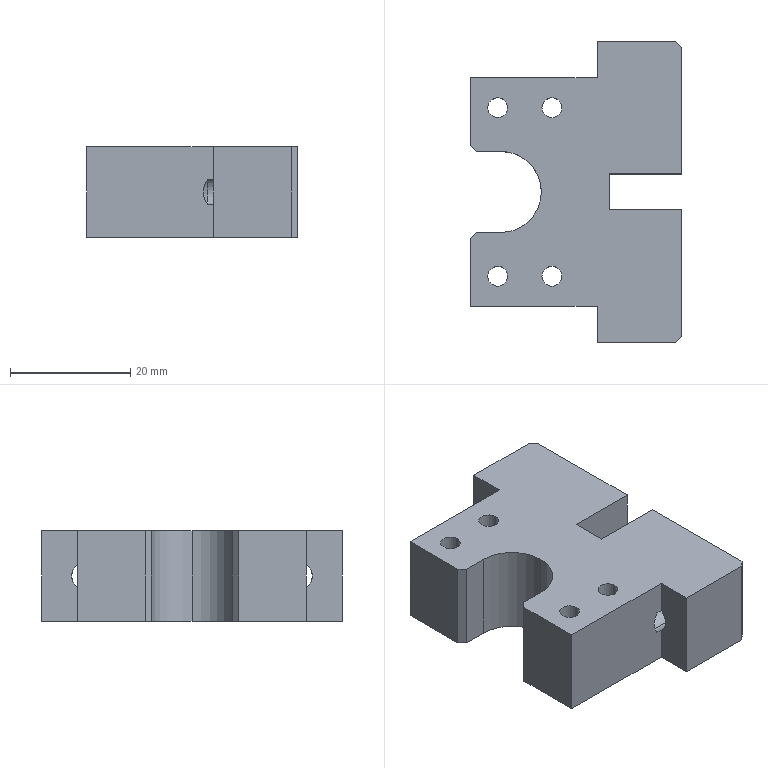Part | SolidWorks | features HoleWzd 3, Chamfer 2, ICE 2, Cut 1, Extrusion 1 | 1 solid | 39 faces | box 35 x 50 x 15 mm | volume 18159 mm3 | plane 21 | cylinder 14 | cone 4 | commonest cylinder face diameters 3.3 x8 5 x4 13.5 x2
STEP:
#1=CARTESIAN_POINT('',(2.5,-17.5,2.5));
#2=VERTEX_POINT('',#1);
#3=CARTESIAN_POINT('',(2.5,-19.,2.));
#4=VERTEX_POINT('',#3);
#5=CARTESIAN_POINT('',(2.5,-17.5,0.));
#6=DIRECTION('',(1.,0.,0.));
#7=DIRECTION('',(0.,0.,-1.));
#8=AXIS2_PLACEMENT_3D('',#5,#6,#7);
#9=CIRCLE('',#8,2.5);
#10=EDGE_CURVE('',#2,#4,#9,.T.);
#11=ORIENTED_EDGE('',*,*,#10,.F.);
#12=CARTESIAN_POINT('',(17.5,-17.5,2.5));
#13=VERTEX_POINT('',#12);
#14=CARTESIAN_POINT('',(17.5,-17.5,2.5));
#15=DIRECTION('',(1.,0.,0.));
#16=VECTOR('',#15,1000.);
#17=LINE('',#14,#16);
#18=EDGE_CURVE('',#2,#13,#17,.T.);
#19=ORIENTED_EDGE('',*,*,#18,.T.);
#20=CARTESIAN_POINT('',(17.5,-17.5,-2.5));
#21=VERTEX_POINT('',#20);
#22=CARTESIAN_POINT('',(17.5,-17.5,0.));
#23=DIRECTION('',(1.,0.,0.));
#24=DIRECTION('',(0.,0.,-1.));
#25=AXIS2_PLACEMENT_3D('',#22,#23,#24);
#26=CIRCLE('',#25,2.5);
#27=EDGE_CURVE('',#13,#21,#26,.T.);
#28=ORIENTED_EDGE('',*,*,#27,.T.);
#29=CARTESIAN_POINT('',(2.5,-17.5,-2.5));
#30=VERTEX_POINT('',#29);
#31=CARTESIAN_POINT('',(17.5,-17.5,-2.5));
#32=DIRECTION('',(1.,0.,0.));
#33=VECTOR('',#32,1000.);
#34=LINE('',#31,#33);
#35=EDGE_CURVE('',#30,#21,#34,.T.);
#36=ORIENTED_EDGE('',*,*,#35,.F.);
#37=CARTESIAN_POINT('',(2.5,-19.,-2.));
#38=VERTEX_POINT('',#37);
#39=CARTESIAN_POINT('',(2.5,-17.5,0.));
#40=DIRECTION('',(1.,0.,0.));
#41=DIRECTION('',(0.,0.,-1.));
#42=AXIS2_PLACEMENT_3D('',#39,#40,#41);
#43=CIRCLE('',#42,2.5);
#44=EDGE_CURVE('',#38,#30,#43,.T.);
#45=ORIENTED_EDGE('',*,*,#44,.F.);
#46=CARTESIAN_POINT('',(3.5,-19.,-2.));
#47=VERTEX_POINT('',#46);
#48=CARTESIAN_POINT('',(17.5,-19.,-2.));
#49=DIRECTION('',(1.,0.,0.));
#50=VECTOR('',#49,1000.);
#51=LINE('',#48,#50);
#52=EDGE_CURVE('',#38,#47,#51,.T.);
#53=ORIENTED_EDGE('',*,*,#52,.T.);
#54=CARTESIAN_POINT('',(3.5,-19.,2.));
#55=VERTEX_POINT('',#54);
#56=CARTESIAN_POINT('',(3.5,-17.5,0.));
#57=DIRECTION('',(-1.,0.,0.));
#58=DIRECTION('',(0.,0.,-1.));
#59=AXIS2_PLACEMENT_3D('',#56,#57,#58);
#60=CIRCLE('',#59,2.5);
#61=EDGE_CURVE('',#47,#55,#60,.T.);
#62=ORIENTED_EDGE('',*,*,#61,.T.);
#63=CARTESIAN_POINT('',(17.5,-19.,2.));
#64=DIRECTION('',(-1.,0.,0.));
#65=VECTOR('',#64,1000.);
#66=LINE('',#63,#65);
#67=EDGE_CURVE('',#55,#4,#66,.T.);
#68=ORIENTED_EDGE('',*,*,#67,.T.);
#69=EDGE_LOOP('',(#11,#19,#28,#36,#45,#53,#62,#68));
#70=FACE_OUTER_BOUND('',#69,.T.);
#71=CARTESIAN_POINT('',(17.5,-17.5,0.));
#72=DIRECTION('',(1.,0.,0.));
#73=DIRECTION('',(0.,0.,-1.));
#74=AXIS2_PLACEMENT_3D('',#71,#72,#73);
#75=CYLINDRICAL_SURFACE('',#74,2.5);
#76=ADVANCED_FACE('',(#70),#75,.F.);
#77=CARTESIAN_POINT('',(0.9978,-17.5,0.));
#78=VERTEX_POINT('',#77);
#79=CARTESIAN_POINT('',(2.5,-17.5,-2.5));
#80=DIRECTION('',(0.515,0.,-0.8572));
#81=VECTOR('',#80,1000.);
#82=LINE('',#79,#81);
#83=EDGE_CURVE('',#78,#30,#82,.T.);
#84=ORIENTED_EDGE('',*,*,#83,.F.);
#85=CARTESIAN_POINT('',(2.5,-17.5,2.5));
#86=DIRECTION('',(0.515,0.,0.8572));
#87=VECTOR('',#86,1000.);
#88=LINE('',#85,#87);
#89=EDGE_CURVE('',#78,#2,#88,.T.);
#90=ORIENTED_EDGE('',*,*,#89,.T.);
#91=ORIENTED_EDGE('',*,*,#10,.T.);
#92=CARTESIAN_POINT('',(2.5,-19.,2.));
#93=CARTESIAN_POINT('',(2.348,-19.,1.683));
#94=CARTESIAN_POINT('',(2.204,-19.,1.361));
#95=CARTESIAN_POINT('',(1.978,-19.,0.6968));
#96=CARTESIAN_POINT('',(1.899,-19.,0.3477));
#97=CARTESIAN_POINT('',(1.899,-19.,-0.1759));
#98=CARTESIAN_POINT('',(1.919,-19.,-0.3531));
#99=CARTESIAN_POINT('',(1.987,-19.,-0.698));
#100=CARTESIAN_POINT('',(2.035,-19.,-0.866));
#101=CARTESIAN_POINT('',(2.204,-19.,-1.362));
#102=CARTESIAN_POINT('',(2.348,-19.,-1.684));
#103=CARTESIAN_POINT('',(2.5,-19.,-2.));
#104=B_SPLINE_CURVE_WITH_KNOTS('',3,(#92,#93,#94,#95,#96,#97,#98,#99,#100,#101,#102,#103),.UNSPECIFIED.,.F.,.F.,(4,2,2,2,2,4),(0.006568,0.007624,0.008679,0.009206,0.009734,0.01079),.UNSPECIFIED.);
#105=EDGE_CURVE('',#4,#38,#104,.T.);
#106=ORIENTED_EDGE('',*,*,#105,.T.);
#107=ORIENTED_EDGE('',*,*,#44,.T.);
#108=EDGE_LOOP('',(#84,#90,#91,#106,#107));
#109=FACE_OUTER_BOUND('',#108,.T.);
#110=CARTESIAN_POINT('',(2.5,-17.5,0.));
#111=DIRECTION('',(1.,0.,0.));
#112=DIRECTION('',(0.,0.,-1.));
#113=AXIS2_PLACEMENT_3D('',#110,#111,#112);
#114=CONICAL_SURFACE('',#113,2.5,1.03);
#115=ADVANCED_FACE('',(#109),#114,.F.);
#116=CARTESIAN_POINT('',(2.5,17.5,2.5));
#117=VERTEX_POINT('',#116);
#118=CARTESIAN_POINT('',(2.5,17.5,-2.5));
#119=VERTEX_POINT('',#118);
#120=CARTESIAN_POINT('',(2.5,17.5,0.));
#121=DIRECTION('',(1.,0.,0.));
#122=DIRECTION('',(0.,0.,-1.));
#123=AXIS2_PLACEMENT_3D('',#120,#121,#122);
#124=CIRCLE('',#123,2.5);
#125=EDGE_CURVE('',#117,#119,#124,.T.);
#126=ORIENTED_EDGE('',*,*,#125,.F.);
#127=CARTESIAN_POINT('',(17.5,17.5,2.5));
#128=VERTEX_POINT('',#127);
#129=CARTESIAN_POINT('',(17.5,17.5,2.5));
#130=DIRECTION('',(1.,0.,0.));
#131=VECTOR('',#130,1000.);
#132=LINE('',#129,#131);
#133=EDGE_CURVE('',#117,#128,#132,.T.);
#134=ORIENTED_EDGE('',*,*,#133,.T.);
#135=CARTESIAN_POINT('',(17.5,17.5,-2.5));
#136=VERTEX_POINT('',#135);
#137=CARTESIAN_POINT('',(17.5,17.5,0.));
#138=DIRECTION('',(1.,0.,0.));
#139=DIRECTION('',(0.,0.,-1.));
#140=AXIS2_PLACEMENT_3D('',#137,#138,#139);
#141=CIRCLE('',#140,2.5);
#142=EDGE_CURVE('',#128,#136,#141,.T.);
#143=ORIENTED_EDGE('',*,*,#142,.T.);
#144=CARTESIAN_POINT('',(17.5,17.5,-2.5));
#145=DIRECTION('',(1.,0.,0.));
#146=VECTOR('',#145,1000.);
#147=LINE('',#144,#146);
#148=EDGE_CURVE('',#119,#136,#147,.T.);
#149=ORIENTED_EDGE('',*,*,#148,.F.);
#150=EDGE_LOOP('',(#126,#134,#143,#149));
#151=FACE_OUTER_BOUND('',#150,.T.);
#152=CARTESIAN_POINT('',(17.5,17.5,0.));
#153=DIRECTION('',(1.,0.,0.));
#154=DIRECTION('',(0.,0.,-1.));
#155=AXIS2_PLACEMENT_3D('',#152,#153,#154);
#156=CYLINDRICAL_SURFACE('',#155,2.5);
#157=ADVANCED_FACE('',(#151),#156,.F.);
#158=CARTESIAN_POINT('',(0.9978,17.5,0.));
#159=VERTEX_POINT('',#158);
#160=CARTESIAN_POINT('',(2.5,17.5,-2.5));
#161=DIRECTION('',(0.515,0.,-0.8572));
#162=VECTOR('',#161,1000.);
#163=LINE('',#160,#162);
#164=EDGE_CURVE('',#159,#119,#163,.T.);
#165=ORIENTED_EDGE('',*,*,#164,.F.);
#166=CARTESIAN_POINT('',(2.5,17.5,2.5));
#167=DIRECTION('',(0.515,0.,0.8572));
#168=VECTOR('',#167,1000.);
#169=LINE('',#166,#168);
#170=EDGE_CURVE('',#159,#117,#169,.T.);
#171=ORIENTED_EDGE('',*,*,#170,.T.);
#172=ORIENTED_EDGE('',*,*,#125,.T.);
#173=EDGE_LOOP('',(#165,#171,#172));
#174=FACE_OUTER_BOUND('',#173,.T.);
#175=CARTESIAN_POINT('',(2.5,17.5,0.));
#176=DIRECTION('',(1.,0.,0.));
#177=DIRECTION('',(0.,0.,-1.));
#178=AXIS2_PLACEMENT_3D('',#175,#176,#177);
#179=CONICAL_SURFACE('',#178,2.5,1.03);
#180=ADVANCED_FACE('',(#174),#179,.F.);
#181=CARTESIAN_POINT('',(-2.35,-14.,7.5));
#182=VERTEX_POINT('',#181);
#183=CARTESIAN_POINT('',(-5.65,-14.,7.5));
#184=VERTEX_POINT('',#183);
#185=CARTESIAN_POINT('',(-4.,-14.,7.5));
#186=DIRECTION('',(0.,0.,-1.));
#187=DIRECTION('',(-1.,0.,0.));
#188=AXIS2_PLACEMENT_3D('',#185,#186,#187);
#189=CIRCLE('',#188,1.65);
#190=EDGE_CURVE('',#182,#184,#189,.T.);
#191=ORIENTED_EDGE('',*,*,#190,.F.);
#192=CARTESIAN_POINT('',(-2.35,-14.,-7.5));
#193=VERTEX_POINT('',#192);
#194=CARTESIAN_POINT('',(-2.35,-14.,-7.5));
#195=DIRECTION('',(0.,0.,-1.));
#196=VECTOR('',#195,1000.);
#197=LINE('',#194,#196);
#198=EDGE_CURVE('',#182,#193,#197,.T.);
#199=ORIENTED_EDGE('',*,*,#198,.T.);
#200=CARTESIAN_POINT('',(-5.65,-14.,-7.5));
#201=VERTEX_POINT('',#200);
#202=CARTESIAN_POINT('',(-4.,-14.,-7.5));
#203=DIRECTION('',(0.,0.,-1.));
#204=DIRECTION('',(-1.,0.,0.));
#205=AXIS2_PLACEMENT_3D('',#202,#203,#204);
#206=CIRCLE('',#205,1.65);
#207=EDGE_CURVE('',#193,#201,#206,.T.);
#208=ORIENTED_EDGE('',*,*,#207,.T.);
#209=CARTESIAN_POINT('',(-5.65,-14.,-7.5));
#210=DIRECTION('',(0.,0.,-1.));
#211=VECTOR('',#210,1000.);
#212=LINE('',#209,#211);
#213=EDGE_CURVE('',#184,#201,#212,.T.);
#214=ORIENTED_EDGE('',*,*,#213,.F.);
#215=EDGE_LOOP('',(#191,#199,#208,#214));
#216=FACE_OUTER_BOUND('',#215,.T.);
#217=CARTESIAN_POINT('',(-4.,-14.,-7.5));
#218=DIRECTION('',(0.,0.,-1.));
#219=DIRECTION('',(-1.,0.,0.));
#220=AXIS2_PLACEMENT_3D('',#217,#218,#219);
#221=CYLINDRICAL_SURFACE('',#220,1.65);
#222=ADVANCED_FACE('',(#216),#221,.F.);
#223=CARTESIAN_POINT('',(-11.35,-14.,7.5));
#224=VERTEX_POINT('',#223);
#225=CARTESIAN_POINT('',(-14.65,-14.,7.5));
#226=VERTEX_POINT('',#225);
#227=CARTESIAN_POINT('',(-13.,-14.,7.5));
#228=DIRECTION('',(0.,0.,-1.));
#229=DIRECTION('',(-1.,0.,0.));
#230=AXIS2_PLACEMENT_3D('',#227,#228,#229);
#231=CIRCLE('',#230,1.65);
#232=EDGE_CURVE('',#224,#226,#231,.T.);
#233=ORIENTED_EDGE('',*,*,#232,.F.);
#234=CARTESIAN_POINT('',(-11.35,-14.,-7.5));
#235=VERTEX_POINT('',#234);
#236=CARTESIAN_POINT('',(-11.35,-14.,-7.5));
#237=DIRECTION('',(0.,0.,-1.));
#238=VECTOR('',#237,1000.);
#239=LINE('',#236,#238);
#240=EDGE_CURVE('',#224,#235,#239,.T.);
#241=ORIENTED_EDGE('',*,*,#240,.T.);
#242=CARTESIAN_POINT('',(-14.65,-14.,-7.5));
#243=VERTEX_POINT('',#242);
#244=CARTESIAN_POINT('',(-13.,-14.,-7.5));
#245=DIRECTION('',(0.,0.,-1.));
#246=DIRECTION('',(-1.,0.,0.));
#247=AXIS2_PLACEMENT_3D('',#244,#245,#246);
#248=CIRCLE('',#247,1.65);
#249=EDGE_CURVE('',#235,#243,#248,.T.);
#250=ORIENTED_EDGE('',*,*,#249,.T.);
#251=CARTESIAN_POINT('',(-14.65,-14.,-7.5));
#252=DIRECTION('',(0.,0.,-1.));
#253=VECTOR('',#252,1000.);
#254=LINE('',#251,#253);
#255=EDGE_CURVE('',#226,#243,#254,.T.);
#256=ORIENTED_EDGE('',*,*,#255,.F.);
#257=EDGE_LOOP('',(#233,#241,#250,#256));
#258=FACE_OUTER_BOUND('',#257,.T.);
#259=CARTESIAN_POINT('',(-13.,-14.,-7.5));
#260=DIRECTION('',(0.,0.,-1.));
#261=DIRECTION('',(-1.,0.,0.));
#262=AXIS2_PLACEMENT_3D('',#259,#260,#261);
#263=CYLINDRICAL_SURFACE('',#262,1.65);
#264=ADVANCED_FACE('',(#258),#263,.F.);
#265=CARTESIAN_POINT('',(-2.35,14.,7.5));
#266=VERTEX_POINT('',#265);
#267=CARTESIAN_POINT('',(-5.65,14.,7.5));
#268=VERTEX_POINT('',#267);
#269=CARTESIAN_POINT('',(-4.,14.,7.5));
#270=DIRECTION('',(0.,0.,-1.));
#271=DIRECTION('',(-1.,0.,0.));
#272=AXIS2_PLACEMENT_3D('',#269,#270,#271);
#273=CIRCLE('',#272,1.65);
#274=EDGE_CURVE('',#266,#268,#273,.T.);
#275=ORIENTED_EDGE('',*,*,#274,.F.);
#276=CARTESIAN_POINT('',(-2.35,14.,-7.5));
#277=VERTEX_POINT('',#276);
#278=CARTESIAN_POINT('',(-2.35,14.,-7.5));
#279=DIRECTION('',(0.,0.,-1.));
#280=VECTOR('',#279,1000.);
#281=LINE('',#278,#280);
#282=EDGE_CURVE('',#266,#277,#281,.T.);
#283=ORIENTED_EDGE('',*,*,#282,.T.);
#284=CARTESIAN_POINT('',(-5.65,14.,-7.5));
#285=VERTEX_POINT('',#284);
#286=CARTESIAN_POINT('',(-4.,14.,-7.5));
#287=DIRECTION('',(0.,0.,-1.));
#288=DIRECTION('',(-1.,0.,0.));
#289=AXIS2_PLACEMENT_3D('',#286,#287,#288);
#290=CIRCLE('',#289,1.65);
#291=EDGE_CURVE('',#277,#285,#290,.T.);
#292=ORIENTED_EDGE('',*,*,#291,.T.);
#293=CARTESIAN_POINT('',(-5.65,14.,-7.5));
#294=DIRECTION('',(0.,0.,-1.));
#295=VECTOR('',#294,1000.);
#296=LINE('',#293,#295);
#297=EDGE_CURVE('',#268,#285,#296,.T.);
#298=ORIENTED_EDGE('',*,*,#297,.F.);
#299=EDGE_LOOP('',(#275,#283,#292,#298));
#300=FACE_OUTER_BOUND('',#299,.T.);
#301=CARTESIAN_POINT('',(-4.,14.,-7.5));
#302=DIRECTION('',(0.,0.,-1.));
#303=DIRECTION('',(-1.,0.,0.));
#304=AXIS2_PLACEMENT_3D('',#301,#302,#303);
#305=CYLINDRICAL_SURFACE('',#304,1.65);
#306=ADVANCED_FACE('',(#300),#305,.F.);
#307=CARTESIAN_POINT('',(-11.35,14.,7.5));
#308=VERTEX_POINT('',#307);
#309=CARTESIAN_POINT('',(-14.65,14.,7.5));
#310=VERTEX_POINT('',#309);
#311=CARTESIAN_POINT('',(-13.,14.,7.5));
#312=DIRECTION('',(0.,0.,-1.));
#313=DIRECTION('',(-1.,0.,0.));
#314=AXIS2_PLACEMENT_3D('',#311,#312,#313);
#315=CIRCLE('',#314,1.65);
#316=EDGE_CURVE('',#308,#310,#315,.T.);
#317=ORIENTED_EDGE('',*,*,#316,.F.);
#318=CARTESIAN_POINT('',(-11.35,14.,-7.5));
#319=VERTEX_POINT('',#318);
#320=CARTESIAN_POINT('',(-11.35,14.,-7.5));
#321=DIRECTION('',(0.,0.,-1.));
#322=VECTOR('',#321,1000.);
#323=LINE('',#320,#322);
#324=EDGE_CURVE('',#308,#319,#323,.T.);
#325=ORIENTED_EDGE('',*,*,#324,.T.);
#326=CARTESIAN_POINT('',(-14.65,14.,-7.5));
#327=VERTEX_POINT('',#326);
#328=CARTESIAN_POINT('',(-13.,14.,-7.5));
#329=DIRECTION('',(0.,0.,-1.));
#330=DIRECTION('',(-1.,0.,0.));
#331=AXIS2_PLACEMENT_3D('',#328,#329,#330);
#332=CIRCLE('',#331,1.65);
#333=EDGE_CURVE('',#319,#327,#332,.T.);
#334=ORIENTED_EDGE('',*,*,#333,.T.);
#335=CARTESIAN_POINT('',(-14.65,14.,-7.5));
#336=DIRECTION('',(0.,0.,-1.));
#337=VECTOR('',#336,1000.);
#338=LINE('',#335,#337);
#339=EDGE_CURVE('',#310,#327,#338,.T.);
#340=ORIENTED_EDGE('',*,*,#339,.F.);
#341=EDGE_LOOP('',(#317,#325,#334,#340));
#342=FACE_OUTER_BOUND('',#341,.T.);
#343=CARTESIAN_POINT('',(-13.,14.,-7.5));
#344=DIRECTION('',(0.,0.,-1.));
#345=DIRECTION('',(-1.,0.,0.));
#346=AXIS2_PLACEMENT_3D('',#343,#344,#345);
#347=CYLINDRICAL_SURFACE('',#346,1.65);
#348=ADVANCED_FACE('',(#342),#347,.F.);
#349=CARTESIAN_POINT('',(-5.75,0.,-7.5));
#350=VERTEX_POINT('',#349);
#351=CARTESIAN_POINT('',(-12.5,6.75,-7.5));
#352=VERTEX_POINT('',#351);
#353=CARTESIAN_POINT('',(-12.5,0.,-7.5));
#354=DIRECTION('',(0.,0.,1.));
#355=DIRECTION('',(1.,0.,0.));
#356=AXIS2_PLACEMENT_3D('',#353,#354,#355);
#357=CIRCLE('',#356,6.75);
#358=EDGE_CURVE('',#350,#352,#357,.T.);
#359=ORIENTED_EDGE('',*,*,#358,.F.);
#360=CARTESIAN_POINT('',(-5.75,0.,7.5));
#361=VERTEX_POINT('',#360);
#362=CARTESIAN_POINT('',(-5.75,0.,-7.5));
#363=DIRECTION('',(0.,0.,1.));
#364=VECTOR('',#363,1000.);
#365=LINE('',#362,#364);
#366=EDGE_CURVE('',#350,#361,#365,.T.);
#367=ORIENTED_EDGE('',*,*,#366,.T.);
#368=CARTESIAN_POINT('',(-12.5,6.75,7.5));
#369=VERTEX_POINT('',#368);
#370=CARTESIAN_POINT('',(-12.5,0.,7.5));
#371=DIRECTION('',(0.,0.,1.));
#372=DIRECTION('',(1.,0.,0.));
#373=AXIS2_PLACEMENT_3D('',#370,#371,#372);
#374=CIRCLE('',#373,6.75);
#375=EDGE_CURVE('',#361,#369,#374,.T.);
#376=ORIENTED_EDGE('',*,*,#375,.T.);
#377=CARTESIAN_POINT('',(-12.5,6.75,-7.5));
#378=DIRECTION('',(0.,0.,1.));
#379=VECTOR('',#378,1000.);
#380=LINE('',#377,#379);
#381=EDGE_CURVE('',#352,#369,#380,.T.);
#382=ORIENTED_EDGE('',*,*,#381,.F.);
#383=EDGE_LOOP('',(#359,#367,#376,#382));
#384=FACE_OUTER_BOUND('',#383,.T.);
#385=CARTESIAN_POINT('',(-12.5,0.,-7.5));
#386=DIRECTION('',(0.,0.,1.));
#387=DIRECTION('',(1.,0.,0.));
#388=AXIS2_PLACEMENT_3D('',#385,#386,#387);
#389=CYLINDRICAL_SURFACE('',#388,6.75);
#390=ADVANCED_FACE('',(#384),#389,.F.);
#391=CARTESIAN_POINT('',(17.5,-17.5,0.));
#392=DIRECTION('',(1.,0.,0.));
#393=DIRECTION('',(0.,0.,-1.));
#394=AXIS2_PLACEMENT_3D('',#391,#392,#393);
#395=CIRCLE('',#394,2.5);
#396=EDGE_CURVE('',#21,#13,#395,.T.);
#397=ORIENTED_EDGE('',*,*,#396,.F.);
#398=ORIENTED_EDGE('',*,*,#27,.F.);
#399=EDGE_LOOP('',(#397,#398));
#400=FACE_BOUND('',#399,.T.);
#401=CARTESIAN_POINT('',(17.5,-24.,-7.5));
#402=VERTEX_POINT('',#401);
#403=CARTESIAN_POINT('',(17.5,-3.,-7.5));
#404=VERTEX_POINT('',#403);
#405=CARTESIAN_POINT('',(17.5,-25.,-7.5));
#406=DIRECTION('',(0.,1.,0.));
#407=VECTOR('',#406,1000.);
#408=LINE('',#405,#407);
#409=EDGE_CURVE('',#402,#404,#408,.T.);
#410=ORIENTED_EDGE('',*,*,#409,.T.);
#411=CARTESIAN_POINT('',(17.5,-3.,7.5));
#412=VERTEX_POINT('',#411);
#413=CARTESIAN_POINT('',(17.5,-3.,-7.5));
#414=DIRECTION('',(0.,0.,1.));
#415=VECTOR('',#414,1000.);
#416=LINE('',#413,#415);
#417=EDGE_CURVE('',#404,#412,#416,.T.);
#418=ORIENTED_EDGE('',*,*,#417,.T.);
#419=CARTESIAN_POINT('',(17.5,-24.,7.5));
#420=VERTEX_POINT('',#419);
#421=CARTESIAN_POINT('',(17.5,-25.,7.5));
#422=DIRECTION('',(0.,1.,0.));
#423=VECTOR('',#422,1000.);
#424=LINE('',#421,#423);
#425=EDGE_CURVE('',#420,#412,#424,.T.);
#426=ORIENTED_EDGE('',*,*,#425,.F.);
#427=CARTESIAN_POINT('',(17.5,-24.,7.5));
#428=DIRECTION('',(0.,0.,-1.));
#429=VECTOR('',#428,1000.);
#430=LINE('',#427,#429);
#431=EDGE_CURVE('',#420,#402,#430,.T.);
#432=ORIENTED_EDGE('',*,*,#431,.T.);
#433=EDGE_LOOP('',(#410,#418,#426,#432));
#434=FACE_OUTER_BOUND('',#433,.T.);
#435=CARTESIAN_POINT('',(17.5,-25.,7.5));
#436=DIRECTION('',(-1.,0.,0.));
#437=DIRECTION('',(0.,0.,1.));
#438=AXIS2_PLACEMENT_3D('',#435,#436,#437);
#439=PLANE('',#438);
#440=ADVANCED_FACE('',(#400,#434),#439,.F.);
#441=CARTESIAN_POINT('',(-17.5,19.,7.5));
#442=VERTEX_POINT('',#441);
#443=CARTESIAN_POINT('',(-17.5,7.75,7.5));
#444=VERTEX_POINT('',#443);
#445=CARTESIAN_POINT('',(-17.5,-25.,7.5));
#446=DIRECTION('',(0.,-1.,0.));
#447=VECTOR('',#446,1000.);
#448=LINE('',#445,#447);
#449=EDGE_CURVE('',#442,#444,#448,.T.);
#450=ORIENTED_EDGE('',*,*,#449,.F.);
#451=CARTESIAN_POINT('',(-17.5,19.,-7.5));
#452=VERTEX_POINT('',#451);
#453=CARTESIAN_POINT('',(-17.5,19.,-7.5));
#454=DIRECTION('',(0.,0.,1.));
#455=VECTOR('',#454,1000.);
#456=LINE('',#453,#455);
#457=EDGE_CURVE('',#452,#442,#456,.T.);
#458=ORIENTED_EDGE('',*,*,#457,.F.);
#459=CARTESIAN_POINT('',(-17.5,7.75,-7.5));
#460=VERTEX_POINT('',#459);
#461=CARTESIAN_POINT('',(-17.5,-25.,-7.5));
#462=DIRECTION('',(0.,-1.,0.));
#463=VECTOR('',#462,1000.);
#464=LINE('',#461,#463);
#465=EDGE_CURVE('',#452,#460,#464,.T.);
#466=ORIENTED_EDGE('',*,*,#465,.T.);
#467=CARTESIAN_POINT('',(-17.5,7.75,7.5));
#468=DIRECTION('',(0.,0.,1.));
#469=VECTOR('',#468,1000.);
#470=LINE('',#467,#469);
#471=EDGE_CURVE('',#460,#444,#470,.T.);
#472=ORIENTED_EDGE('',*,*,#471,.T.);
#473=EDGE_LOOP('',(#450,#458,#466,#472));
#474=FACE_OUTER_BOUND('',#473,.T.);
#475=CARTESIAN_POINT('',(-17.5,-25.,7.5));
#476=DIRECTION('',(1.,0.,0.));
#477=DIRECTION('',(0.,0.,-1.));
#478=AXIS2_PLACEMENT_3D('',#475,#476,#477);
#479=PLANE('',#478);
#480=ADVANCED_FACE('',(#474),#479,.F.);
#481=CARTESIAN_POINT('',(17.5,17.5,0.));
#482=DIRECTION('',(1.,0.,0.));
#483=DIRECTION('',(0.,0.,-1.));
#484=AXIS2_PLACEMENT_3D('',#481,#482,#483);
#485=CIRCLE('',#484,2.5);
#486=EDGE_CURVE('',#136,#128,#485,.T.);
#487=ORIENTED_EDGE('',*,*,#486,.F.);
#488=ORIENTED_EDGE('',*,*,#142,.F.);
#489=EDGE_LOOP('',(#487,#488));
#490=FACE_BOUND('',#489,.T.);
#491=CARTESIAN_POINT('',(17.5,3.,7.5));
#492=VERTEX_POINT('',#491);
#493=CARTESIAN_POINT('',(17.5,24.,7.5));
#494=VERTEX_POINT('',#493);
#495=CARTESIAN_POINT('',(17.5,-25.,7.5));
#496=DIRECTION('',(0.,1.,0.));
#497=VECTOR('',#496,1000.);
#498=LINE('',#495,#497);
#499=EDGE_CURVE('',#492,#494,#498,.T.);
#500=ORIENTED_EDGE('',*,*,#499,.F.);
#501=CARTESIAN_POINT('',(17.5,3.,-7.5));
#502=VERTEX_POINT('',#501);
#503=CARTESIAN_POINT('',(17.5,3.,-7.5));
#504=DIRECTION('',(0.,0.,1.));
#505=VECTOR('',#504,1000.);
#506=LINE('',#503,#505);
#507=EDGE_CURVE('',#502,#492,#506,.T.);
#508=ORIENTED_EDGE('',*,*,#507,.F.);
#509=CARTESIAN_POINT('',(17.5,24.,-7.5));
#510=VERTEX_POINT('',#509);
#511=CARTESIAN_POINT('',(17.5,-25.,-7.5));
#512=DIRECTION('',(0.,1.,0.));
#513=VECTOR('',#512,1000.);
#514=LINE('',#511,#513);
#515=EDGE_CURVE('',#502,#510,#514,.T.);
#516=ORIENTED_EDGE('',*,*,#515,.T.);
#517=CARTESIAN_POINT('',(17.5,24.,7.5));
#518=DIRECTION('',(0.,0.,1.));
#519=VECTOR('',#518,1000.);
#520=LINE('',#517,#519);
#521=EDGE_CURVE('',#510,#494,#520,.T.);
#522=ORIENTED_EDGE('',*,*,#521,.T.);
#523=EDGE_LOOP('',(#500,#508,#516,#522));
#524=FACE_OUTER_BOUND('',#523,.T.);
#525=CARTESIAN_POINT('',(17.5,-25.,7.5));
#526=DIRECTION('',(-1.,0.,0.));
#527=DIRECTION('',(0.,0.,1.));
#528=AXIS2_PLACEMENT_3D('',#525,#526,#527);
#529=PLANE('',#528);
#530=ADVANCED_FACE('',(#490,#524),#529,.F.);
#531=CARTESIAN_POINT('',(16.5,25.,-7.5));
#532=VERTEX_POINT('',#531);
#533=CARTESIAN_POINT('',(3.5,25.,-7.5));
#534=VERTEX_POINT('',#533);
#535=CARTESIAN_POINT('',(-17.5,25.,-7.5));
#536=DIRECTION('',(-1.,0.,0.));
#537=VECTOR('',#536,1000.);
#538=LINE('',#535,#537);
#539=EDGE_CURVE('',#532,#534,#538,.T.);
#540=ORIENTED_EDGE('',*,*,#539,.T.);
#541=CARTESIAN_POINT('',(3.5,25.,7.5));
#542=VERTEX_POINT('',#541);
#543=CARTESIAN_POINT('',(3.5,25.,-7.5));
#544=DIRECTION('',(0.,0.,1.));
#545=VECTOR('',#544,1000.);
#546=LINE('',#543,#545);
#547=EDGE_CURVE('',#534,#542,#546,.T.);
#548=ORIENTED_EDGE('',*,*,#547,.T.);
#549=CARTESIAN_POINT('',(16.5,25.,7.5));
#550=VERTEX_POINT('',#549);
#551=CARTESIAN_POINT('',(-17.5,25.,7.5));
#552=DIRECTION('',(-1.,0.,0.));
#553=VECTOR('',#552,1000.);
#554=LINE('',#551,#553);
#555=EDGE_CURVE('',#550,#542,#554,.T.);
#556=ORIENTED_EDGE('',*,*,#555,.F.);
#557=CARTESIAN_POINT('',(16.5,25.,7.5));
#558=DIRECTION('',(0.,0.,-1.));
#559=VECTOR('',#558,1000.);
#560=LINE('',#557,#559);
#561=EDGE_CURVE('',#550,#532,#560,.T.);
#562=ORIENTED_EDGE('',*,*,#561,.T.);
#563=EDGE_LOOP('',(#540,#548,#556,#562));
#564=FACE_OUTER_BOUND('',#563,.T.);
#565=CARTESIAN_POINT('',(-17.5,25.,7.5));
#566=DIRECTION('',(0.,-1.,0.));
#567=DIRECTION('',(0.,0.,-1.));
#568=AXIS2_PLACEMENT_3D('',#565,#566,#567);
#569=PLANE('',#568);
#570=ADVANCED_FACE('',(#564),#569,.F.);
#571=CARTESIAN_POINT('',(-17.5,-7.75,-7.5));
#572=VERTEX_POINT('',#571);
#573=CARTESIAN_POINT('',(-17.5,-19.,-7.5));
#574=VERTEX_POINT('',#573);
#575=CARTESIAN_POINT('',(-17.5,-25.,-7.5));
#576=DIRECTION('',(0.,-1.,0.));
#577=VECTOR('',#576,1000.);
#578=LINE('',#575,#577);
#579=EDGE_CURVE('',#572,#574,#578,.T.);
#580=ORIENTED_EDGE('',*,*,#579,.T.);
#581=CARTESIAN_POINT('',(-17.5,-19.,7.5));
#582=VERTEX_POINT('',#581);
#583=CARTESIAN_POINT('',(-17.5,-19.,-7.5));
#584=DIRECTION('',(0.,0.,1.));
#585=VECTOR('',#584,1000.);
#586=LINE('',#583,#585);
#587=EDGE_CURVE('',#574,#582,#586,.T.);
#588=ORIENTED_EDGE('',*,*,#587,.T.);
#589=CARTESIAN_POINT('',(-17.5,-7.75,7.5));
#590=VERTEX_POINT('',#589);
#591=CARTESIAN_POINT('',(-17.5,-25.,7.5));
#592=DIRECTION('',(0.,-1.,0.));
#593=VECTOR('',#592,1000.);
#594=LINE('',#591,#593);
#595=EDGE_CURVE('',#590,#582,#594,.T.);
#596=ORIENTED_EDGE('',*,*,#595,.F.);
#597=CARTESIAN_POINT('',(-17.5,-7.75,7.5));
#598=DIRECTION('',(0.,0.,-1.));
#599=VECTOR('',#598,1000.);
#600=LINE('',#597,#599);
#601=EDGE_CURVE('',#590,#572,#600,.T.);
#602=ORIENTED_EDGE('',*,*,#601,.T.);
#603=EDGE_LOOP('',(#580,#588,#596,#602));
#604=FACE_OUTER_BOUND('',#603,.T.);
#605=CARTESIAN_POINT('',(-17.5,-25.,7.5));
#606=DIRECTION('',(1.,0.,0.));
#607=DIRECTION('',(0.,0.,-1.));
#608=AXIS2_PLACEMENT_3D('',#605,#606,#607);
#609=PLANE('',#608);
#610=ADVANCED_FACE('',(#604),#609,.F.);
#611=CARTESIAN_POINT('',(3.5,-25.,7.5));
#612=VERTEX_POINT('',#611);
#613=CARTESIAN_POINT('',(16.5,-25.,7.5));
#614=VERTEX_POINT('',#613);
#615=CARTESIAN_POINT('',(-17.5,-25.,7.5));
#616=DIRECTION('',(1.,0.,0.));
#617=VECTOR('',#616,1000.);
#618=LINE('',#615,#617);
#619=EDGE_CURVE('',#612,#614,#618,.T.);
#620=ORIENTED_EDGE('',*,*,#619,.F.);
#621=CARTESIAN_POINT('',(3.5,-25.,-7.5));
#622=VERTEX_POINT('',#621);
#623=CARTESIAN_POINT('',(3.5,-25.,-7.5));
#624=DIRECTION('',(0.,0.,1.));
#625=VECTOR('',#624,1000.);
#626=LINE('',#623,#625);
#627=EDGE_CURVE('',#622,#612,#626,.T.);
#628=ORIENTED_EDGE('',*,*,#627,.F.);
#629=CARTESIAN_POINT('',(16.5,-25.,-7.5));
#630=VERTEX_POINT('',#629);
#631=CARTESIAN_POINT('',(-17.5,-25.,-7.5));
#632=DIRECTION('',(1.,0.,0.));
#633=VECTOR('',#632,1000.);
#634=LINE('',#631,#633);
#635=EDGE_CURVE('',#622,#630,#634,.T.);
#636=ORIENTED_EDGE('',*,*,#635,.T.);
#637=CARTESIAN_POINT('',(16.5,-25.,7.5));
#638=DIRECTION('',(0.,0.,1.));
#639=VECTOR('',#638,1000.);
#640=LINE('',#637,#639);
#641=EDGE_CURVE('',#630,#614,#640,.T.);
#642=ORIENTED_EDGE('',*,*,#641,.T.);
#643=EDGE_LOOP('',(#620,#628,#636,#642));
#644=FACE_OUTER_BOUND('',#643,.T.);
#645=CARTESIAN_POINT('',(-17.5,-25.,7.5));
#646=DIRECTION('',(0.,1.,0.));
#647=DIRECTION('',(0.,0.,1.));
#648=AXIS2_PLACEMENT_3D('',#645,#646,#647);
#649=PLANE('',#648);
#650=ADVANCED_FACE('',(#644),#649,.F.);
#651=CARTESIAN_POINT('',(-4.,-14.,7.5));
#652=DIRECTION('',(0.,0.,-1.));
#653=DIRECTION('',(-1.,0.,0.));
#654=AXIS2_PLACEMENT_3D('',#651,#652,#653);
#655=CIRCLE('',#654,1.65);
#656=EDGE_CURVE('',#184,#182,#655,.T.);
#657=ORIENTED_EDGE('',*,*,#656,.T.);
#658=ORIENTED_EDGE('',*,*,#190,.T.);
#659=EDGE_LOOP('',(#657,#658));
#660=FACE_BOUND('',#659,.T.);
#661=CARTESIAN_POINT('',(-13.,-14.,7.5));
#662=DIRECTION('',(0.,0.,-1.));
#663=DIRECTION('',(-1.,0.,0.));
#664=AXIS2_PLACEMENT_3D('',#661,#662,#663);
#665=CIRCLE('',#664,1.65);
#666=EDGE_CURVE('',#226,#224,#665,.T.);
#667=ORIENTED_EDGE('',*,*,#666,.T.);
#668=ORIENTED_EDGE('',*,*,#232,.T.);
#669=EDGE_LOOP('',(#667,#668));
#670=FACE_BOUND('',#669,.T.);
#671=CARTESIAN_POINT('',(-4.,14.,7.5));
#672=DIRECTION('',(0.,0.,-1.));
#673=DIRECTION('',(-1.,0.,0.));
#674=AXIS2_PLACEMENT_3D('',#671,#672,#673);
#675=CIRCLE('',#674,1.65);
#676=EDGE_CURVE('',#268,#266,#675,.T.);
#677=ORIENTED_EDGE('',*,*,#676,.T.);
#678=ORIENTED_EDGE('',*,*,#274,.T.);
#679=EDGE_LOOP('',(#677,#678));
#680=FACE_BOUND('',#679,.T.);
#681=CARTESIAN_POINT('',(-13.,14.,7.5));
#682=DIRECTION('',(0.,0.,-1.));
#683=DIRECTION('',(-1.,0.,0.));
#684=AXIS2_PLACEMENT_3D('',#681,#682,#683);
#685=CIRCLE('',#684,1.65);
#686=EDGE_CURVE('',#310,#308,#685,.T.);
#687=ORIENTED_EDGE('',*,*,#686,.T.);
#688=ORIENTED_EDGE('',*,*,#316,.T.);
#689=EDGE_LOOP('',(#687,#688));
#690=FACE_BOUND('',#689,.T.);
#691=ORIENTED_EDGE('',*,*,#595,.T.);
#692=CARTESIAN_POINT('',(3.5,-19.,7.5));
#693=VERTEX_POINT('',#692);
#694=CARTESIAN_POINT('',(-17.5,-19.,7.5));
#695=DIRECTION('',(-1.,0.,0.));
#696=VECTOR('',#695,1000.);
#697=LINE('',#694,#696);
#698=EDGE_CURVE('',#693,#582,#697,.T.);
#699=ORIENTED_EDGE('',*,*,#698,.F.);
#700=CARTESIAN_POINT('',(3.5,-25.,7.5));
#701=DIRECTION('',(0.,1.,0.));
#702=VECTOR('',#701,1000.);
#703=LINE('',#700,#702);
#704=EDGE_CURVE('',#612,#693,#703,.T.);
#705=ORIENTED_EDGE('',*,*,#704,.F.);
#706=ORIENTED_EDGE('',*,*,#619,.T.);
#707=CARTESIAN_POINT('',(17.5,-24.,7.5));
#708=DIRECTION('',(0.7071,0.7071,0.));
#709=VECTOR('',#708,1000.);
#710=LINE('',#707,#709);
#711=EDGE_CURVE('',#614,#420,#710,.T.);
#712=ORIENTED_EDGE('',*,*,#711,.T.);
#713=ORIENTED_EDGE('',*,*,#425,.T.);
#714=CARTESIAN_POINT('',(5.5,-3.,7.5));
#715=VERTEX_POINT('',#714);
#716=CARTESIAN_POINT('',(5.5,-3.,7.5));
#717=DIRECTION('',(1.,0.,0.));
#718=VECTOR('',#717,1000.);
#719=LINE('',#716,#718);
#720=EDGE_CURVE('',#715,#412,#719,.T.);
#721=ORIENTED_EDGE('',*,*,#720,.F.);
#722=CARTESIAN_POINT('',(5.5,3.,7.5));
#723=VERTEX_POINT('',#722);
#724=CARTESIAN_POINT('',(5.5,3.,7.5));
#725=DIRECTION('',(0.,-1.,0.));
#726=VECTOR('',#725,1000.);
#727=LINE('',#724,#726);
#728=EDGE_CURVE('',#723,#715,#727,.T.);
#729=ORIENTED_EDGE('',*,*,#728,.F.);
#730=CARTESIAN_POINT('',(5.5,3.,7.5));
#731=DIRECTION('',(-1.,0.,0.));
#732=VECTOR('',#731,1000.);
#733=LINE('',#730,#732);
#734=EDGE_CURVE('',#492,#723,#733,.T.);
#735=ORIENTED_EDGE('',*,*,#734,.F.);
#736=ORIENTED_EDGE('',*,*,#499,.T.);
#737=CARTESIAN_POINT('',(16.5,25.,7.5));
#738=DIRECTION('',(-0.7071,0.7071,0.));
#739=VECTOR('',#738,1000.);
#740=LINE('',#737,#739);
#741=EDGE_CURVE('',#494,#550,#740,.T.);
#742=ORIENTED_EDGE('',*,*,#741,.T.);
#743=ORIENTED_EDGE('',*,*,#555,.T.);
#744=CARTESIAN_POINT('',(3.5,19.,7.5));
#745=VERTEX_POINT('',#744);
#746=CARTESIAN_POINT('',(3.5,19.,7.5));
#747=DIRECTION('',(0.,1.,0.));
#748=VECTOR('',#747,1000.);
#749=LINE('',#746,#748);
#750=EDGE_CURVE('',#745,#542,#749,.T.);
#751=ORIENTED_EDGE('',*,*,#750,.F.);
#752=CARTESIAN_POINT('',(-17.5,19.,7.5));
#753=DIRECTION('',(1.,0.,0.));
#754=VECTOR('',#753,1000.);
#755=LINE('',#752,#754);
#756=EDGE_CURVE('',#442,#745,#755,.T.);
#757=ORIENTED_EDGE('',*,*,#756,.F.);
#758=ORIENTED_EDGE('',*,*,#449,.T.);
#759=CARTESIAN_POINT('',(-16.5,6.75,7.5));
#760=VERTEX_POINT('',#759);
#761=CARTESIAN_POINT('',(-17.5,7.75,7.5));
#762=DIRECTION('',(0.7071,-0.7071,0.));
#763=VECTOR('',#762,1000.);
#764=LINE('',#761,#763);
#765=EDGE_CURVE('',#444,#760,#764,.T.);
#766=ORIENTED_EDGE('',*,*,#765,.T.);
#767=CARTESIAN_POINT('',(-17.5,6.75,7.5));
#768=DIRECTION('',(-1.,0.,0.));
#769=VECTOR('',#768,1000.);
#770=LINE('',#767,#769);
#771=EDGE_CURVE('',#369,#760,#770,.T.);
#772=ORIENTED_EDGE('',*,*,#771,.F.);
#773=ORIENTED_EDGE('',*,*,#375,.F.);
#774=CARTESIAN_POINT('',(-12.5,-6.75,7.5));
#775=VERTEX_POINT('',#774);
#776=CARTESIAN_POINT('',(-12.5,0.,7.5));
#777=DIRECTION('',(0.,0.,1.));
#778=DIRECTION('',(1.,0.,0.));
#779=AXIS2_PLACEMENT_3D('',#776,#777,#778);
#780=CIRCLE('',#779,6.75);
#781=EDGE_CURVE('',#775,#361,#780,.T.);
#782=ORIENTED_EDGE('',*,*,#781,.F.);
#783=CARTESIAN_POINT('',(-16.5,-6.75,7.5));
#784=VERTEX_POINT('',#783);
#785=CARTESIAN_POINT('',(-17.5,-6.75,7.5));
#786=DIRECTION('',(1.,0.,0.));
#787=VECTOR('',#786,1000.);
#788=LINE('',#785,#787);
#789=EDGE_CURVE('',#784,#775,#788,.T.);
#790=ORIENTED_EDGE('',*,*,#789,.F.);
#791=CARTESIAN_POINT('',(-16.5,-6.75,7.5));
#792=DIRECTION('',(-0.7071,-0.7071,0.));
#793=VECTOR('',#792,1000.);
#794=LINE('',#791,#793);
#795=EDGE_CURVE('',#784,#590,#794,.T.);
#796=ORIENTED_EDGE('',*,*,#795,.T.);
#797=EDGE_LOOP('',(#691,#699,#705,#706,#712,#713,#721,#729,#735,#736,#742,#743,#751,#757,#758,#766,#772,#773,#782,#790,#796));
#798=FACE_OUTER_BOUND('',#797,.T.);
#799=CARTESIAN_POINT('',(0.,0.,7.5));
#800=DIRECTION('',(0.,0.,-1.));
#801=DIRECTION('',(-1.,0.,0.));
#802=AXIS2_PLACEMENT_3D('',#799,#800,#801);
#803=PLANE('',#802);
#804=ADVANCED_FACE('',(#660,#670,#680,#690,#798),#803,.F.);
#805=CARTESIAN_POINT('',(3.5,-19.,-7.5));
#806=VERTEX_POINT('',#805);
#807=CARTESIAN_POINT('',(-17.5,-19.,-7.5));
#808=DIRECTION('',(-1.,0.,0.));
#809=VECTOR('',#808,1000.);
#810=LINE('',#807,#809);
#811=EDGE_CURVE('',#806,#574,#810,.T.);
#812=ORIENTED_EDGE('',*,*,#811,.T.);
#813=ORIENTED_EDGE('',*,*,#579,.F.);
#814=CARTESIAN_POINT('',(-16.5,-6.75,-7.5));
#815=VERTEX_POINT('',#814);
#816=CARTESIAN_POINT('',(-4.875,4.875,-7.5));
#817=DIRECTION('',(0.7071,0.7071,0.));
#818=VECTOR('',#817,1000.);
#819=LINE('',#816,#818);
#820=EDGE_CURVE('',#572,#815,#819,.T.);
#821=ORIENTED_EDGE('',*,*,#820,.T.);
#822=CARTESIAN_POINT('',(-12.5,-6.75,-7.5));
#823=VERTEX_POINT('',#822);
#824=CARTESIAN_POINT('',(-17.5,-6.75,-7.5));
#825=DIRECTION('',(1.,0.,0.));
#826=VECTOR('',#825,1000.);
#827=LINE('',#824,#826);
#828=EDGE_CURVE('',#815,#823,#827,.T.);
#829=ORIENTED_EDGE('',*,*,#828,.T.);
#830=CARTESIAN_POINT('',(-12.5,0.,-7.5));
#831=DIRECTION('',(0.,0.,1.));
#832=DIRECTION('',(1.,0.,0.));
#833=AXIS2_PLACEMENT_3D('',#830,#831,#832);
#834=CIRCLE('',#833,6.75);
#835=EDGE_CURVE('',#823,#350,#834,.T.);
#836=ORIENTED_EDGE('',*,*,#835,.T.);
#837=ORIENTED_EDGE('',*,*,#358,.T.);
#838=CARTESIAN_POINT('',(-16.5,6.75,-7.5));
#839=VERTEX_POINT('',#838);
#840=CARTESIAN_POINT('',(-17.5,6.75,-7.5));
#841=DIRECTION('',(-1.,0.,0.));
#842=VECTOR('',#841,1000.);
#843=LINE('',#840,#842);
#844=EDGE_CURVE('',#352,#839,#843,.T.);
#845=ORIENTED_EDGE('',*,*,#844,.T.);
#846=CARTESIAN_POINT('',(-4.875,-4.875,-7.5));
#847=DIRECTION('',(-0.7071,0.7071,0.));
#848=VECTOR('',#847,1000.);
#849=LINE('',#846,#848);
#850=EDGE_CURVE('',#839,#460,#849,.T.);
#851=ORIENTED_EDGE('',*,*,#850,.T.);
#852=ORIENTED_EDGE('',*,*,#465,.F.);
#853=CARTESIAN_POINT('',(3.5,19.,-7.5));
#854=VERTEX_POINT('',#853);
#855=CARTESIAN_POINT('',(-17.5,19.,-7.5));
#856=DIRECTION('',(1.,0.,0.));
#857=VECTOR('',#856,1000.);
#858=LINE('',#855,#857);
#859=EDGE_CURVE('',#452,#854,#858,.T.);
#860=ORIENTED_EDGE('',*,*,#859,.T.);
#861=CARTESIAN_POINT('',(3.5,19.,-7.5));
#862=DIRECTION('',(0.,1.,0.));
#863=VECTOR('',#862,1000.);
#864=LINE('',#861,#863);
#865=EDGE_CURVE('',#854,#534,#864,.T.);
#866=ORIENTED_EDGE('',*,*,#865,.T.);
#867=ORIENTED_EDGE('',*,*,#539,.F.);
#868=CARTESIAN_POINT('',(20.75,20.75,-7.5));
#869=DIRECTION('',(0.7071,-0.7071,0.));
#870=VECTOR('',#869,1000.);
#871=LINE('',#868,#870);
#872=EDGE_CURVE('',#532,#510,#871,.T.);
#873=ORIENTED_EDGE('',*,*,#872,.T.);
#874=ORIENTED_EDGE('',*,*,#515,.F.);
#875=CARTESIAN_POINT('',(5.5,3.,-7.5));
#876=VERTEX_POINT('',#875);
#877=CARTESIAN_POINT('',(5.5,3.,-7.5));
#878=DIRECTION('',(-1.,0.,0.));
#879=VECTOR('',#878,1000.);
#880=LINE('',#877,#879);
#881=EDGE_CURVE('',#502,#876,#880,.T.);
#882=ORIENTED_EDGE('',*,*,#881,.T.);
#883=CARTESIAN_POINT('',(5.5,-3.,-7.5));
#884=VERTEX_POINT('',#883);
#885=CARTESIAN_POINT('',(5.5,3.,-7.5));
#886=DIRECTION('',(0.,-1.,0.));
#887=VECTOR('',#886,1000.);
#888=LINE('',#885,#887);
#889=EDGE_CURVE('',#876,#884,#888,.T.);
#890=ORIENTED_EDGE('',*,*,#889,.T.);
#891=CARTESIAN_POINT('',(5.5,-3.,-7.5));
#892=DIRECTION('',(1.,0.,0.));
#893=VECTOR('',#892,1000.);
#894=LINE('',#891,#893);
#895=EDGE_CURVE('',#884,#404,#894,.T.);
#896=ORIENTED_EDGE('',*,*,#895,.T.);
#897=ORIENTED_EDGE('',*,*,#409,.F.);
#898=CARTESIAN_POINT('',(20.75,-20.75,-7.5));
#899=DIRECTION('',(-0.7071,-0.7071,0.));
#900=VECTOR('',#899,1000.);
#901=LINE('',#898,#900);
#902=EDGE_CURVE('',#402,#630,#901,.T.);
#903=ORIENTED_EDGE('',*,*,#902,.T.);
#904=ORIENTED_EDGE('',*,*,#635,.F.);
#905=CARTESIAN_POINT('',(3.5,-25.,-7.5));
#906=DIRECTION('',(0.,1.,0.));
#907=VECTOR('',#906,1000.);
#908=LINE('',#905,#907);
#909=EDGE_CURVE('',#622,#806,#908,.T.);
#910=ORIENTED_EDGE('',*,*,#909,.T.);
#911=EDGE_LOOP('',(#812,#813,#821,#829,#836,#837,#845,#851,#852,#860,#866,#867,#873,#874,#882,#890,#896,#897,#903,#904,#910));
#912=FACE_OUTER_BOUND('',#911,.T.);
#913=CARTESIAN_POINT('',(-4.,-14.,-7.5));
#914=DIRECTION('',(0.,0.,-1.));
#915=DIRECTION('',(-1.,0.,0.));
#916=AXIS2_PLACEMENT_3D('',#913,#914,#915);
#917=CIRCLE('',#916,1.65);
#918=EDGE_CURVE('',#201,#193,#917,.T.);
#919=ORIENTED_EDGE('',*,*,#918,.F.);
#920=ORIENTED_EDGE('',*,*,#207,.F.);
#921=EDGE_LOOP('',(#919,#920));
#922=FACE_BOUND('',#921,.T.);
#923=CARTESIAN_POINT('',(-13.,-14.,-7.5));
#924=DIRECTION('',(0.,0.,-1.));
#925=DIRECTION('',(-1.,0.,0.));
#926=AXIS2_PLACEMENT_3D('',#923,#924,#925);
#927=CIRCLE('',#926,1.65);
#928=EDGE_CURVE('',#243,#235,#927,.T.);
#929=ORIENTED_EDGE('',*,*,#928,.F.);
#930=ORIENTED_EDGE('',*,*,#249,.F.);
#931=EDGE_LOOP('',(#929,#930));
#932=FACE_BOUND('',#931,.T.);
#933=CARTESIAN_POINT('',(-4.,14.,-7.5));
#934=DIRECTION('',(0.,0.,-1.));
#935=DIRECTION('',(-1.,0.,0.));
#936=AXIS2_PLACEMENT_3D('',#933,#934,#935);
#937=CIRCLE('',#936,1.65);
#938=EDGE_CURVE('',#285,#277,#937,.T.);
#939=ORIENTED_EDGE('',*,*,#938,.F.);
#940=ORIENTED_EDGE('',*,*,#291,.F.);
#941=EDGE_LOOP('',(#939,#940));
#942=FACE_BOUND('',#941,.T.);
#943=CARTESIAN_POINT('',(-13.,14.,-7.5));
#944=DIRECTION('',(0.,0.,-1.));
#945=DIRECTION('',(-1.,0.,0.));
#946=AXIS2_PLACEMENT_3D('',#943,#944,#945);
#947=CIRCLE('',#946,1.65);
#948=EDGE_CURVE('',#327,#319,#947,.T.);
#949=ORIENTED_EDGE('',*,*,#948,.F.);
#950=ORIENTED_EDGE('',*,*,#333,.F.);
#951=EDGE_LOOP('',(#949,#950));
#952=FACE_BOUND('',#951,.T.);
#953=CARTESIAN_POINT('',(0.,0.,-7.5));
#954=DIRECTION('',(0.,0.,-1.));
#955=DIRECTION('',(-1.,0.,0.));
#956=AXIS2_PLACEMENT_3D('',#953,#954,#955);
#957=PLANE('',#956);
#958=ADVANCED_FACE('',(#912,#922,#932,#942,#952),#957,.T.);
#959=ORIENTED_EDGE('',*,*,#771,.T.);
#960=CARTESIAN_POINT('',(-16.5,6.75,-7.5));
#961=DIRECTION('',(0.,0.,-1.));
#962=VECTOR('',#961,1000.);
#963=LINE('',#960,#962);
#964=EDGE_CURVE('',#760,#839,#963,.T.);
#965=ORIENTED_EDGE('',*,*,#964,.T.);
#966=ORIENTED_EDGE('',*,*,#844,.F.);
#967=ORIENTED_EDGE('',*,*,#381,.T.);
#968=EDGE_LOOP('',(#959,#965,#966,#967));
#969=FACE_OUTER_BOUND('',#968,.T.);
#970=CARTESIAN_POINT('',(-17.5,6.75,-7.5));
#971=DIRECTION('',(0.,1.,0.));
#972=DIRECTION('',(0.,0.,1.));
#973=AXIS2_PLACEMENT_3D('',#970,#971,#972);
#974=PLANE('',#973);
#975=ADVANCED_FACE('',(#969),#974,.F.);
#976=ORIENTED_EDGE('',*,*,#366,.F.);
#977=ORIENTED_EDGE('',*,*,#835,.F.);
#978=CARTESIAN_POINT('',(-12.5,-6.75,-7.5));
#979=DIRECTION('',(0.,0.,1.));
#980=VECTOR('',#979,1000.);
#981=LINE('',#978,#980);
#982=EDGE_CURVE('',#823,#775,#981,.T.);
#983=ORIENTED_EDGE('',*,*,#982,.T.);
#984=ORIENTED_EDGE('',*,*,#781,.T.);
#985=EDGE_LOOP('',(#976,#977,#983,#984));
#986=FACE_OUTER_BOUND('',#985,.T.);
#987=CARTESIAN_POINT('',(-12.5,0.,-7.5));
#988=DIRECTION('',(0.,0.,1.));
#989=DIRECTION('',(1.,0.,0.));
#990=AXIS2_PLACEMENT_3D('',#987,#988,#989);
#991=CYLINDRICAL_SURFACE('',#990,6.75);
#992=ADVANCED_FACE('',(#986),#991,.F.);
#993=ORIENTED_EDGE('',*,*,#828,.F.);
#994=CARTESIAN_POINT('',(-16.5,-6.75,-7.5));
#995=DIRECTION('',(0.,0.,1.));
#996=VECTOR('',#995,1000.);
#997=LINE('',#994,#996);
#998=EDGE_CURVE('',#815,#784,#997,.T.);
#999=ORIENTED_EDGE('',*,*,#998,.T.);
#1000=ORIENTED_EDGE('',*,*,#789,.T.);
#1001=ORIENTED_EDGE('',*,*,#982,.F.);
#1002=EDGE_LOOP('',(#993,#999,#1000,#1001));
#1003=FACE_OUTER_BOUND('',#1002,.T.);
#1004=CARTESIAN_POINT('',(-17.5,-6.75,-7.5));
#1005=DIRECTION('',(0.,-1.,0.));
#1006=DIRECTION('',(0.,0.,-1.));
#1007=AXIS2_PLACEMENT_3D('',#1004,#1005,#1006);
#1008=PLANE('',#1007);
#1009=ADVANCED_FACE('',(#1003),#1008,.F.);
#1010=ORIENTED_EDGE('',*,*,#324,.F.);
#1011=ORIENTED_EDGE('',*,*,#686,.F.);
#1012=ORIENTED_EDGE('',*,*,#339,.T.);
#1013=ORIENTED_EDGE('',*,*,#948,.T.);
#1014=EDGE_LOOP('',(#1010,#1011,#1012,#1013));
#1015=FACE_OUTER_BOUND('',#1014,.T.);
#1016=CARTESIAN_POINT('',(-13.,14.,-7.5));
#1017=DIRECTION('',(0.,0.,-1.));
#1018=DIRECTION('',(-1.,0.,0.));
#1019=AXIS2_PLACEMENT_3D('',#1016,#1017,#1018);
#1020=CYLINDRICAL_SURFACE('',#1019,1.65);
#1021=ADVANCED_FACE('',(#1015),#1020,.F.);
#1022=ORIENTED_EDGE('',*,*,#282,.F.);
#1023=ORIENTED_EDGE('',*,*,#676,.F.);
#1024=ORIENTED_EDGE('',*,*,#297,.T.);
#1025=ORIENTED_EDGE('',*,*,#938,.T.);
#1026=EDGE_LOOP('',(#1022,#1023,#1024,#1025));
#1027=FACE_OUTER_BOUND('',#1026,.T.);
#1028=CARTESIAN_POINT('',(-4.,14.,-7.5));
#1029=DIRECTION('',(0.,0.,-1.));
#1030=DIRECTION('',(-1.,0.,0.));
#1031=AXIS2_PLACEMENT_3D('',#1028,#1029,#1030);
#1032=CYLINDRICAL_SURFACE('',#1031,1.65);
#1033=ADVANCED_FACE('',(#1027),#1032,.F.);
#1034=ORIENTED_EDGE('',*,*,#240,.F.);
#1035=ORIENTED_EDGE('',*,*,#666,.F.);
#1036=ORIENTED_EDGE('',*,*,#255,.T.);
#1037=ORIENTED_EDGE('',*,*,#928,.T.);
#1038=EDGE_LOOP('',(#1034,#1035,#1036,#1037));
#1039=FACE_OUTER_BOUND('',#1038,.T.);
#1040=CARTESIAN_POINT('',(-13.,-14.,-7.5));
#1041=DIRECTION('',(0.,0.,-1.));
#1042=DIRECTION('',(-1.,0.,0.));
#1043=AXIS2_PLACEMENT_3D('',#1040,#1041,#1042);
#1044=CYLINDRICAL_SURFACE('',#1043,1.65);
#1045=ADVANCED_FACE('',(#1039),#1044,.F.);
#1046=ORIENTED_EDGE('',*,*,#198,.F.);
#1047=ORIENTED_EDGE('',*,*,#656,.F.);
#1048=ORIENTED_EDGE('',*,*,#213,.T.);
#1049=ORIENTED_EDGE('',*,*,#918,.T.);
#1050=EDGE_LOOP('',(#1046,#1047,#1048,#1049));
#1051=FACE_OUTER_BOUND('',#1050,.T.);
#1052=CARTESIAN_POINT('',(-4.,-14.,-7.5));
#1053=DIRECTION('',(0.,0.,-1.));
#1054=DIRECTION('',(-1.,0.,0.));
#1055=AXIS2_PLACEMENT_3D('',#1052,#1053,#1054);
#1056=CYLINDRICAL_SURFACE('',#1055,1.65);
#1057=ADVANCED_FACE('',(#1051),#1056,.F.);
#1058=ORIENTED_EDGE('',*,*,#741,.F.);
#1059=ORIENTED_EDGE('',*,*,#521,.F.);
#1060=ORIENTED_EDGE('',*,*,#872,.F.);
#1061=ORIENTED_EDGE('',*,*,#561,.F.);
#1062=EDGE_LOOP('',(#1058,#1059,#1060,#1061));
#1063=FACE_OUTER_BOUND('',#1062,.T.);
#1064=CARTESIAN_POINT('',(16.5,25.,7.5));
#1065=DIRECTION('',(-0.7071,-0.7071,0.));
#1066=DIRECTION('',(0.,0.,-1.));
#1067=AXIS2_PLACEMENT_3D('',#1064,#1065,#1066);
#1068=PLANE('',#1067);
#1069=ADVANCED_FACE('',(#1063),#1068,.F.);
#1070=ORIENTED_EDGE('',*,*,#711,.F.);
#1071=ORIENTED_EDGE('',*,*,#641,.F.);
#1072=ORIENTED_EDGE('',*,*,#902,.F.);
#1073=ORIENTED_EDGE('',*,*,#431,.F.);
#1074=EDGE_LOOP('',(#1070,#1071,#1072,#1073));
#1075=FACE_OUTER_BOUND('',#1074,.T.);
#1076=CARTESIAN_POINT('',(17.5,-24.,7.5));
#1077=DIRECTION('',(-0.7071,0.7071,0.));
#1078=DIRECTION('',(0.,0.,-1.));
#1079=AXIS2_PLACEMENT_3D('',#1076,#1077,#1078);
#1080=PLANE('',#1079);
#1081=ADVANCED_FACE('',(#1075),#1080,.F.);
#1082=ORIENTED_EDGE('',*,*,#820,.F.);
#1083=ORIENTED_EDGE('',*,*,#601,.F.);
#1084=ORIENTED_EDGE('',*,*,#795,.F.);
#1085=ORIENTED_EDGE('',*,*,#998,.F.);
#1086=EDGE_LOOP('',(#1082,#1083,#1084,#1085));
#1087=FACE_OUTER_BOUND('',#1086,.T.);
#1088=CARTESIAN_POINT('',(-16.5,-6.75,-7.5));
#1089=DIRECTION('',(0.7071,-0.7071,0.));
#1090=DIRECTION('',(0.,0.,1.));
#1091=AXIS2_PLACEMENT_3D('',#1088,#1089,#1090);
#1092=PLANE('',#1091);
#1093=ADVANCED_FACE('',(#1087),#1092,.F.);
#1094=ORIENTED_EDGE('',*,*,#850,.F.);
#1095=ORIENTED_EDGE('',*,*,#964,.F.);
#1096=ORIENTED_EDGE('',*,*,#765,.F.);
#1097=ORIENTED_EDGE('',*,*,#471,.F.);
#1098=EDGE_LOOP('',(#1094,#1095,#1096,#1097));
#1099=FACE_OUTER_BOUND('',#1098,.T.);
#1100=CARTESIAN_POINT('',(-17.5,7.75,7.5));
#1101=DIRECTION('',(0.7071,0.7071,0.));
#1102=DIRECTION('',(0.,0.,1.));
#1103=AXIS2_PLACEMENT_3D('',#1100,#1101,#1102);
#1104=PLANE('',#1103);
#1105=ADVANCED_FACE('',(#1099),#1104,.F.);
#1106=ORIENTED_EDGE('',*,*,#170,.F.);
#1107=ORIENTED_EDGE('',*,*,#164,.T.);
#1108=CARTESIAN_POINT('',(2.5,19.,-2.));
#1109=VERTEX_POINT('',#1108);
#1110=CARTESIAN_POINT('',(2.5,17.5,0.));
#1111=DIRECTION('',(1.,0.,0.));
#1112=DIRECTION('',(0.,0.,-1.));
#1113=AXIS2_PLACEMENT_3D('',#1110,#1111,#1112);
#1114=CIRCLE('',#1113,2.5);
#1115=EDGE_CURVE('',#119,#1109,#1114,.T.);
#1116=ORIENTED_EDGE('',*,*,#1115,.T.);
#1117=CARTESIAN_POINT('',(2.5,19.,2.));
#1118=VERTEX_POINT('',#1117);
#1119=CARTESIAN_POINT('',(2.5,19.,-2.));
#1120=CARTESIAN_POINT('',(2.348,19.,-1.683));
#1121=CARTESIAN_POINT('',(2.204,19.,-1.361));
#1122=CARTESIAN_POINT('',(1.978,19.,-0.6968));
#1123=CARTESIAN_POINT('',(1.899,19.,-0.3477));
#1124=CARTESIAN_POINT('',(1.899,19.,0.1759));
#1125=CARTESIAN_POINT('',(1.919,19.,0.3531));
#1126=CARTESIAN_POINT('',(1.987,19.,0.698));
#1127=CARTESIAN_POINT('',(2.035,19.,0.866));
#1128=CARTESIAN_POINT('',(2.204,19.,1.362));
#1129=CARTESIAN_POINT('',(2.348,19.,1.684));
#1130=CARTESIAN_POINT('',(2.5,19.,2.));
#1131=B_SPLINE_CURVE_WITH_KNOTS('',3,(#1119,#1120,#1121,#1122,#1123,#1124,#1125,#1126,#1127,#1128,#1129,#1130),.UNSPECIFIED.,.F.,.F.,(4,2,2,2,2,4),(0.006568,0.007624,0.008679,0.009206,0.009734,0.01079),.UNSPECIFIED.);
#1132=EDGE_CURVE('',#1109,#1118,#1131,.T.);
#1133=ORIENTED_EDGE('',*,*,#1132,.T.);
#1134=CARTESIAN_POINT('',(2.5,17.5,0.));
#1135=DIRECTION('',(1.,0.,0.));
#1136=DIRECTION('',(0.,0.,-1.));
#1137=AXIS2_PLACEMENT_3D('',#1134,#1135,#1136);
#1138=CIRCLE('',#1137,2.5);
#1139=EDGE_CURVE('',#1118,#117,#1138,.T.);
#1140=ORIENTED_EDGE('',*,*,#1139,.T.);
#1141=EDGE_LOOP('',(#1106,#1107,#1116,#1133,#1140));
#1142=FACE_OUTER_BOUND('',#1141,.T.);
#1143=CARTESIAN_POINT('',(2.5,17.5,0.));
#1144=DIRECTION('',(1.,0.,0.));
#1145=DIRECTION('',(0.,0.,-1.));
#1146=AXIS2_PLACEMENT_3D('',#1143,#1144,#1145);
#1147=CONICAL_SURFACE('',#1146,2.5,1.03);
#1148=ADVANCED_FACE('',(#1142),#1147,.F.);
#1149=ORIENTED_EDGE('',*,*,#133,.F.);
#1150=ORIENTED_EDGE('',*,*,#1139,.F.);
#1151=CARTESIAN_POINT('',(3.5,19.,2.));
#1152=VERTEX_POINT('',#1151);
#1153=CARTESIAN_POINT('',(17.5,19.,2.));
#1154=DIRECTION('',(1.,0.,0.));
#1155=VECTOR('',#1154,1000.);
#1156=LINE('',#1153,#1155);
#1157=EDGE_CURVE('',#1118,#1152,#1156,.T.);
#1158=ORIENTED_EDGE('',*,*,#1157,.T.);
#1159=CARTESIAN_POINT('',(3.5,19.,-2.));
#1160=VERTEX_POINT('',#1159);
#1161=CARTESIAN_POINT('',(3.5,17.5,0.));
#1162=DIRECTION('',(-1.,0.,0.));
#1163=DIRECTION('',(0.,0.,-1.));
#1164=AXIS2_PLACEMENT_3D('',#1161,#1162,#1163);
#1165=CIRCLE('',#1164,2.5);
#1166=EDGE_CURVE('',#1152,#1160,#1165,.T.);
#1167=ORIENTED_EDGE('',*,*,#1166,.T.);
#1168=CARTESIAN_POINT('',(17.5,19.,-2.));
#1169=DIRECTION('',(-1.,0.,0.));
#1170=VECTOR('',#1169,1000.);
#1171=LINE('',#1168,#1170);
#1172=EDGE_CURVE('',#1160,#1109,#1171,.T.);
#1173=ORIENTED_EDGE('',*,*,#1172,.T.);
#1174=ORIENTED_EDGE('',*,*,#1115,.F.);
#1175=ORIENTED_EDGE('',*,*,#148,.T.);
#1176=ORIENTED_EDGE('',*,*,#486,.T.);
#1177=EDGE_LOOP('',(#1149,#1150,#1158,#1167,#1173,#1174,#1175,#1176));
#1178=FACE_OUTER_BOUND('',#1177,.T.);
#1179=CARTESIAN_POINT('',(17.5,17.5,0.));
#1180=DIRECTION('',(1.,0.,0.));
#1181=DIRECTION('',(0.,0.,-1.));
#1182=AXIS2_PLACEMENT_3D('',#1179,#1180,#1181);
#1183=CYLINDRICAL_SURFACE('',#1182,2.5);
#1184=ADVANCED_FACE('',(#1178),#1183,.F.);
#1185=ORIENTED_EDGE('',*,*,#89,.F.);
#1186=ORIENTED_EDGE('',*,*,#83,.T.);
#1187=CARTESIAN_POINT('',(2.5,-17.5,0.));
#1188=DIRECTION('',(1.,0.,0.));
#1189=DIRECTION('',(0.,0.,-1.));
#1190=AXIS2_PLACEMENT_3D('',#1187,#1188,#1189);
#1191=CIRCLE('',#1190,2.5);
#1192=EDGE_CURVE('',#30,#2,#1191,.T.);
#1193=ORIENTED_EDGE('',*,*,#1192,.T.);
#1194=EDGE_LOOP('',(#1185,#1186,#1193));
#1195=FACE_OUTER_BOUND('',#1194,.T.);
#1196=CARTESIAN_POINT('',(2.5,-17.5,0.));
#1197=DIRECTION('',(1.,0.,0.));
#1198=DIRECTION('',(0.,0.,-1.));
#1199=AXIS2_PLACEMENT_3D('',#1196,#1197,#1198);
#1200=CONICAL_SURFACE('',#1199,2.5,1.03);
#1201=ADVANCED_FACE('',(#1195),#1200,.F.);
#1202=ORIENTED_EDGE('',*,*,#18,.F.);
#1203=ORIENTED_EDGE('',*,*,#1192,.F.);
#1204=ORIENTED_EDGE('',*,*,#35,.T.);
#1205=ORIENTED_EDGE('',*,*,#396,.T.);
#1206=EDGE_LOOP('',(#1202,#1203,#1204,#1205));
#1207=FACE_OUTER_BOUND('',#1206,.T.);
#1208=CARTESIAN_POINT('',(17.5,-17.5,0.));
#1209=DIRECTION('',(1.,0.,0.));
#1210=DIRECTION('',(0.,0.,-1.));
#1211=AXIS2_PLACEMENT_3D('',#1208,#1209,#1210);
#1212=CYLINDRICAL_SURFACE('',#1211,2.5);
#1213=ADVANCED_FACE('',(#1207),#1212,.F.);
#1214=ORIENTED_EDGE('',*,*,#720,.T.);
#1215=ORIENTED_EDGE('',*,*,#417,.F.);
#1216=ORIENTED_EDGE('',*,*,#895,.F.);
#1217=CARTESIAN_POINT('',(5.5,-3.,-7.5));
#1218=DIRECTION('',(0.,0.,1.));
#1219=VECTOR('',#1218,1000.);
#1220=LINE('',#1217,#1219);
#1221=EDGE_CURVE('',#884,#715,#1220,.T.);
#1222=ORIENTED_EDGE('',*,*,#1221,.T.);
#1223=EDGE_LOOP('',(#1214,#1215,#1216,#1222));
#1224=FACE_OUTER_BOUND('',#1223,.T.);
#1225=CARTESIAN_POINT('',(5.5,-3.,-7.5));
#1226=DIRECTION('',(0.,-1.,0.));
#1227=DIRECTION('',(0.,0.,-1.));
#1228=AXIS2_PLACEMENT_3D('',#1225,#1226,#1227);
#1229=PLANE('',#1228);
#1230=ADVANCED_FACE('',(#1224),#1229,.F.);
#1231=ORIENTED_EDGE('',*,*,#728,.T.);
#1232=ORIENTED_EDGE('',*,*,#1221,.F.);
#1233=ORIENTED_EDGE('',*,*,#889,.F.);
#1234=CARTESIAN_POINT('',(5.5,3.,-7.5));
#1235=DIRECTION('',(0.,0.,1.));
#1236=VECTOR('',#1235,1000.);
#1237=LINE('',#1234,#1236);
#1238=EDGE_CURVE('',#876,#723,#1237,.T.);
#1239=ORIENTED_EDGE('',*,*,#1238,.T.);
#1240=EDGE_LOOP('',(#1231,#1232,#1233,#1239));
#1241=FACE_OUTER_BOUND('',#1240,.T.);
#1242=CARTESIAN_POINT('',(5.5,3.,-7.5));
#1243=DIRECTION('',(-1.,0.,0.));
#1244=DIRECTION('',(0.,0.,1.));
#1245=AXIS2_PLACEMENT_3D('',#1242,#1243,#1244);
#1246=PLANE('',#1245);
#1247=ADVANCED_FACE('',(#1241),#1246,.F.);
#1248=ORIENTED_EDGE('',*,*,#734,.T.);
#1249=ORIENTED_EDGE('',*,*,#1238,.F.);
#1250=ORIENTED_EDGE('',*,*,#881,.F.);
#1251=ORIENTED_EDGE('',*,*,#507,.T.);
#1252=EDGE_LOOP('',(#1248,#1249,#1250,#1251));
#1253=FACE_OUTER_BOUND('',#1252,.T.);
#1254=CARTESIAN_POINT('',(5.5,3.,-7.5));
#1255=DIRECTION('',(0.,1.,0.));
#1256=DIRECTION('',(0.,0.,1.));
#1257=AXIS2_PLACEMENT_3D('',#1254,#1255,#1256);
#1258=PLANE('',#1257);
#1259=ADVANCED_FACE('',(#1253),#1258,.F.);
#1260=CARTESIAN_POINT('',(3.5,-19.,-7.5));
#1261=DIRECTION('',(0.,0.,1.));
#1262=VECTOR('',#1261,1000.);
#1263=LINE('',#1260,#1262);
#1264=EDGE_CURVE('',#55,#693,#1263,.T.);
#1265=ORIENTED_EDGE('',*,*,#1264,.T.);
#1266=ORIENTED_EDGE('',*,*,#698,.T.);
#1267=ORIENTED_EDGE('',*,*,#587,.F.);
#1268=ORIENTED_EDGE('',*,*,#811,.F.);
#1269=CARTESIAN_POINT('',(3.5,-19.,-7.5));
#1270=DIRECTION('',(0.,0.,1.));
#1271=VECTOR('',#1270,1000.);
#1272=LINE('',#1269,#1271);
#1273=EDGE_CURVE('',#806,#47,#1272,.T.);
#1274=ORIENTED_EDGE('',*,*,#1273,.T.);
#1275=ORIENTED_EDGE('',*,*,#52,.F.);
#1276=ORIENTED_EDGE('',*,*,#105,.F.);
#1277=ORIENTED_EDGE('',*,*,#67,.F.);
#1278=EDGE_LOOP('',(#1265,#1266,#1267,#1268,#1274,#1275,#1276,#1277));
#1279=FACE_OUTER_BOUND('',#1278,.T.);
#1280=CARTESIAN_POINT('',(-17.5,-19.,-7.5));
#1281=DIRECTION('',(0.,1.,0.));
#1282=DIRECTION('',(0.,0.,1.));
#1283=AXIS2_PLACEMENT_3D('',#1280,#1281,#1282);
#1284=PLANE('',#1283);
#1285=ADVANCED_FACE('',(#1279),#1284,.F.);
#1286=ORIENTED_EDGE('',*,*,#1273,.F.);
#1287=ORIENTED_EDGE('',*,*,#909,.F.);
#1288=ORIENTED_EDGE('',*,*,#627,.T.);
#1289=ORIENTED_EDGE('',*,*,#704,.T.);
#1290=ORIENTED_EDGE('',*,*,#1264,.F.);
#1291=ORIENTED_EDGE('',*,*,#61,.F.);
#1292=EDGE_LOOP('',(#1286,#1287,#1288,#1289,#1290,#1291));
#1293=FACE_OUTER_BOUND('',#1292,.T.);
#1294=CARTESIAN_POINT('',(3.5,-25.,-7.5));
#1295=DIRECTION('',(1.,0.,0.));
#1296=DIRECTION('',(0.,0.,-1.));
#1297=AXIS2_PLACEMENT_3D('',#1294,#1295,#1296);
#1298=PLANE('',#1297);
#1299=ADVANCED_FACE('',(#1293),#1298,.F.);
#1300=CARTESIAN_POINT('',(3.5,19.,-7.5));
#1301=DIRECTION('',(0.,0.,1.));
#1302=VECTOR('',#1301,1000.);
#1303=LINE('',#1300,#1302);
#1304=EDGE_CURVE('',#1152,#745,#1303,.T.);
#1305=ORIENTED_EDGE('',*,*,#1304,.T.);
#1306=ORIENTED_EDGE('',*,*,#750,.T.);
#1307=ORIENTED_EDGE('',*,*,#547,.F.);
#1308=ORIENTED_EDGE('',*,*,#865,.F.);
#1309=CARTESIAN_POINT('',(3.5,19.,-7.5));
#1310=DIRECTION('',(0.,0.,1.));
#1311=VECTOR('',#1310,1000.);
#1312=LINE('',#1309,#1311);
#1313=EDGE_CURVE('',#854,#1160,#1312,.T.);
#1314=ORIENTED_EDGE('',*,*,#1313,.T.);
#1315=ORIENTED_EDGE('',*,*,#1166,.F.);
#1316=EDGE_LOOP('',(#1305,#1306,#1307,#1308,#1314,#1315));
#1317=FACE_OUTER_BOUND('',#1316,.T.);
#1318=CARTESIAN_POINT('',(3.5,19.,-7.5));
#1319=DIRECTION('',(1.,0.,0.));
#1320=DIRECTION('',(0.,0.,-1.));
#1321=AXIS2_PLACEMENT_3D('',#1318,#1319,#1320);
#1322=PLANE('',#1321);
#1323=ADVANCED_FACE('',(#1317),#1322,.F.);
#1324=ORIENTED_EDGE('',*,*,#1313,.F.);
#1325=ORIENTED_EDGE('',*,*,#859,.F.);
#1326=ORIENTED_EDGE('',*,*,#457,.T.);
#1327=ORIENTED_EDGE('',*,*,#756,.T.);
#1328=ORIENTED_EDGE('',*,*,#1304,.F.);
#1329=ORIENTED_EDGE('',*,*,#1157,.F.);
#1330=ORIENTED_EDGE('',*,*,#1132,.F.);
#1331=ORIENTED_EDGE('',*,*,#1172,.F.);
#1332=EDGE_LOOP('',(#1324,#1325,#1326,#1327,#1328,#1329,#1330,#1331));
#1333=FACE_OUTER_BOUND('',#1332,.T.);
#1334=CARTESIAN_POINT('',(-17.5,19.,-7.5));
#1335=DIRECTION('',(0.,-1.,0.));
#1336=DIRECTION('',(0.,0.,-1.));
#1337=AXIS2_PLACEMENT_3D('',#1334,#1335,#1336);
#1338=PLANE('',#1337);
#1339=ADVANCED_FACE('',(#1333),#1338,.F.);
#1340=CLOSED_SHELL('',(#76,#115,#157,#180,#222,#264,#306,#348,#390,#440,#480,#530,#570,#610,#650,#804,#958,#975,#992,#1009,#1021,#1033,#1045,#1057,#1069,#1081,#1093,#1105,#1148,#1184,#1201,#1213,#1230,#1247,#1259,#1285,#1299,#1323,#1339));
#1341=MANIFOLD_SOLID_BREP('',#1340);
#1342=CARTESIAN_POINT('',(0.,0.,0.));
#1343=DIRECTION('',(0.,0.,1.));
#1344=DIRECTION('',(1.,0.,0.));
#1345=AXIS2_PLACEMENT_3D('',#1342,#1343,#1344);
#1346=(LENGTH_UNIT()NAMED_UNIT(*)SI_UNIT(.MILLI.,.METRE.));
#1347=UNCERTAINTY_MEASURE_WITH_UNIT(LENGTH_MEASURE(0.00001),#1346,'','');
#1348=(NAMED_UNIT(*)PLANE_ANGLE_UNIT()SI_UNIT($,.RADIAN.));
#1349=(NAMED_UNIT(*)SI_UNIT($,.STERADIAN.)SOLID_ANGLE_UNIT());
#1350=(GEOMETRIC_REPRESENTATION_CONTEXT(3)GLOBAL_UNCERTAINTY_ASSIGNED_CONTEXT((#1347))GLOBAL_UNIT_ASSIGNED_CONTEXT((#1346,#1348,#1349))REPRESENTATION_CONTEXT('',''));
#1351=ADVANCED_BREP_SHAPE_REPRESENTATION('',(#1341,#1345),#1350);